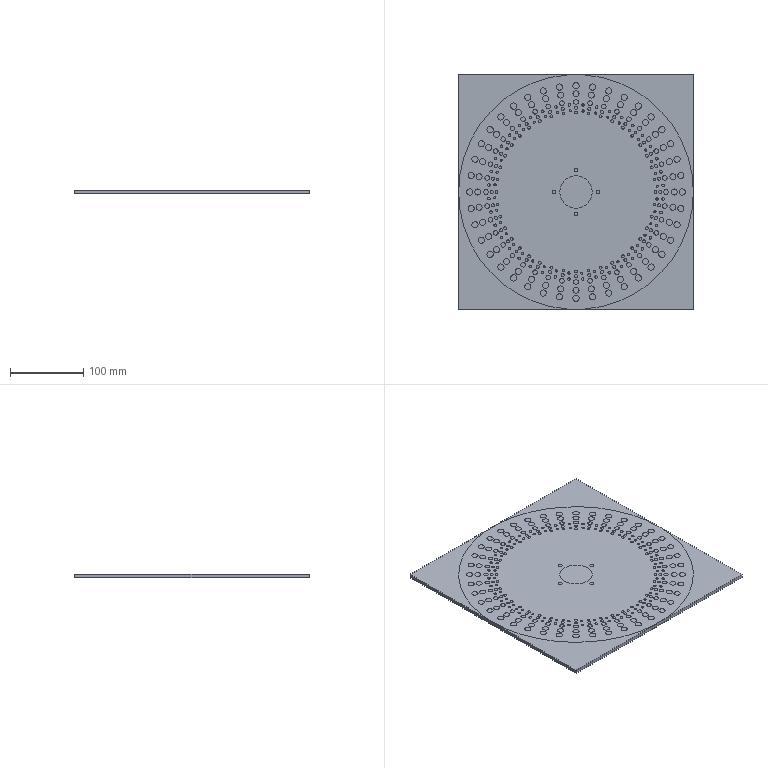NC program | NX | posted with a generic post | part box 320 x 320 x 5 mm
Lines 1 to 986 of 63198:
N10 G17 G21 G94 G90
(等高外形 , TOOL : D17R0.8圆鼻飞刀)
N12 T07 M6
N14 /M1
N16 G54
N18 G17 G0 G90 X-172.144 Y-7.615 S2000 M3
N20 G43 Z20. H7
N22 Z0.4
N24 G94 G1 Z0.2 F1600.
N26 G3 X-168.5 Y0.198 R10.2
N28 G2 X-168.486 Y2.393 R173.905 F2000.
N30 X-168.27 Y8.907 R224.797
N32 X-167.861 Y14.646 R236.128
N34 X-167.519 Y18.143 R188.644
N36 G1 X-167.43 Y18.944
N38 X-167.002 Y22.411
N40 X-166.958 Y22.734
N42 X-166.495 Y25.903
N44 X-166.42 Y26.394
N46 X-165.835 Y29.843
N48 X-165.736 Y30.384
N50 X-165.168 Y33.335
N52 X-165.023 Y34.046
N54 X-164.391 Y36.979
N56 G2 X-163.515 Y40.666 R172.039
N58 G1 X-163.504 Y40.725
N60 X-163.459 Y40.904
N62 X-162.566 Y44.32
N64 X-162.418 Y44.862
N66 X-161.528 Y47.963
N68 X-161.313 Y48.673
N70 X-160.428 Y51.514
N72 X-160.425 Y51.533
N74 X-160.217 Y52.17
N76 X-159.213 Y55.157
N78 X-159.209 Y55.177
N80 X-159.037 Y55.668
N82 X-157.73 Y59.291
N84 G2 X-155.928 Y63.842 R140.951
N86 G1 X-155.204 Y65.595
N88 X-155.198 Y65.614
N90 X-154.966 Y66.16
N92 X-153.672 Y69.114
N94 X-153.425 Y69.657
N96 X-152.087 Y72.536
N98 X-151.847 Y73.038
N100 X-150.456 Y75.861
N102 X-150.226 Y76.316
N104 X-148.47 Y79.688
N106 G2 X-144.35 Y86.927 R201.508
N108 X-141.803 Y91.008 R164.836
N110 X-140.487 Y93.026 R79.908
N112 G1 X-138.909 Y95.369
N114 X-138.905 Y95.38
N116 X-138.553 Y95.888
N118 X-136.686 Y98.533
N120 X-136.302 Y99.063
N122 X-134.557 Y101.416
N124 X-134.553 Y101.426
N126 X-134.36 Y101.682
N128 X-132.184 Y104.496
N130 X-131.82 Y104.954
N132 X-129.826 Y107.411
N134 X-129.462 Y107.85
N136 X-127.434 Y110.234
N138 X-127.424 Y110.25
N140 X-127.013 Y110.722
N142 X-124.939 Y113.058
N144 X-124.477 Y113.567
N146 X-122.385 Y115.818
N148 X-122.119 Y116.1
N150 X-119.721 Y118.569
N152 X-119.438 Y118.856
N154 X-117.036 Y121.22
N156 X-116.873 Y121.378
N158 X-114.328 Y123.778
N160 X-113.958 Y124.119
N162 X-111.454 Y126.372
N164 X-111.044 Y126.733
N166 X-108.684 Y128.759
N168 X-108.672 Y128.772
N170 X-108.129 Y129.228
N172 X-105.763 Y131.171
N174 X-105.423 Y131.445
N176 X-102.869 Y133.449
N178 X-102.857 Y133.462
N180 X-102.3 Y133.89
N182 X-99.77 Y135.786
N184 X-99.386 Y136.068
N186 X-96.741 Y137.959
N188 X-96.26 Y138.297
N190 X-93.619 Y140.095
N192 X-93.612 Y140.103
N194 X-93.228 Y140.358
N196 X-90.47 Y142.151
N198 X-90.059 Y142.412
N200 X-88.008 Y143.688
N202 G2 X-84.044 Y146.042 R227.342
N204 G1 X-83.647 Y146.271
N206 X-80.688 Y147.924
N208 X-80.15 Y148.216
N210 X-77.434 Y149.652
N212 X-76.944 Y149.905
N214 X-73.737 Y151.512
N216 G2 X-69.074 Y153.683 R141.064
N218 G1 X-68.492 Y153.941
N220 X-67.271 Y154.485
N222 X-67.253 Y154.495
N224 X-66.743 Y154.717
N226 X-63.701 Y155.993
N228 X-63.245 Y156.179
N230 X-60.241 Y157.362
N232 X-59.748 Y157.55
N234 X-56.778 Y158.641
N236 X-56.761 Y158.65
N238 X-56.25 Y158.832
N240 X-53.158 Y159.894
N242 X-52.753 Y160.029
N244 X-50.058 Y160.892
N246 X-49.256 Y161.14
N248 X-45.977 Y162.104
N250 G2 X-42.334 Y163.094 R449.314
N252 G1 X-41.678 Y163.263
N254 X-38.634 Y164.008
N256 X-38.62 Y164.014
N258 X-38.303 Y164.088
N260 X-35.011 Y164.821
N262 X-34.392 Y164.952
N264 X-31.367 Y165.55
N266 X-31.35 Y165.556
N268 X-29.346 Y165.924
N270 G2 X-26.349 Y166.42 R109.611
N272 G1 X-25.939 Y166.482
N274 X-23.845 Y166.803
N276 X-23.316 Y166.878
N278 X-20.056 Y167.3
N280 X-19.527 Y167.363
N282 X-16.394 Y167.699
N284 X-16.03 Y167.735
N286 X-12.66 Y168.022
N288 X-11.95 Y168.075
N290 X-8.871 Y168.265
N292 X-8.452 Y168.288
N294 X-5.082 Y168.422
N296 G2 X-0.103 Y168.492 R132.588
N298 G1 X2.496 Y168.48
N300 G2 X5.629 Y168.405 R104.354
N302 X9.91 Y168.207 R298.334
N304 G1 X10.54 Y168.169
N306 X13.716 Y167.937
N308 X13.735 Y167.938
N310 X15.9 Y167.75
N312 G2 X21.203 Y167.159 R243.166
N314 G1 X21.859 Y167.075
N316 X25.011 Y166.632
N318 G2 X28.508 Y166.07 R175.312
N320 G1 X29.364 Y165.921
N322 X32.912 Y165.253
N324 X33.153 Y165.205
N326 X36.068 Y164.593
N328 G2 X39.929 Y163.7 R166.413
N330 G1 X40.513 Y163.554
N332 X43.355 Y162.825
N334 X44.009 Y162.65
N336 X47.759 Y161.596
N338 G2 X51.321 Y160.493 R251.012
N340 G1 X51.338 Y160.485
N342 X54.21 Y159.538
N344 X54.229 Y159.534
N346 X54.502 Y159.441
N348 X57.853 Y158.256
N350 X57.999 Y158.203
N352 X61.943 Y156.708
N354 X64.538 Y155.651
N356 X65.27 Y155.345
N358 X68.247 Y154.059
N360 X68.784 Y153.82
N362 X71.812 Y152.429
N364 X71.989 Y152.347
N366 X75.08 Y150.847
N368 X75.633 Y150.572
N370 X78.413 Y149.139
N372 X78.427 Y149.134
N374 X78.81 Y148.933
N376 X81.67 Y147.38
N378 X81.68 Y147.377
N380 X82.256 Y147.057
N382 X85.644 Y145.119
N384 G2 X91.484 Y141.501 R211.587
N386 G1 X91.808 Y141.292
N388 X94.58 Y139.448
N390 X94.594 Y139.442
N392 G2 X100.72 Y135.083 R200.557
N394 G1 X101.134 Y134.773
N396 X103.711 Y132.8
N398 X104.049 Y132.536
N400 X106.622 Y130.474
N402 X107.11 Y130.075
N404 X109.501 Y128.067
N406 X109.878 Y127.745
N408 X112.372 Y125.557
N410 X112.792 Y125.179
N412 X115.159 Y123.006
N414 X115.483 Y122.702
N416 X117.91 Y120.37
N418 X118.27 Y120.017
N420 X120.552 Y117.724
N422 X120.815 Y117.456
N424 X123.114 Y115.042
N426 G2 X127.737 Y109.878 R173.773
N428 G1 X128.178 Y109.368
N430 X128.189 Y109.359
N432 X128.531 Y108.957
N434 X130.548 Y106.527
N436 X130.563 Y106.514
N438 X130.863 Y106.146
N440 X132.884 Y103.599
N442 X132.897 Y103.586
N444 X133.194 Y103.206
N446 X135.211 Y100.547
N448 X135.526 Y100.124
N450 X137.404 Y97.528
N452 X137.741 Y97.054
N454 X139.608 Y94.345
N456 X139.749 Y94.139
N458 X141.63 Y91.285
N460 X141.938 Y90.805
N462 X143.689 Y88.005
N464 X144.058 Y87.401
N466 X145.535 Y84.913
N468 X145.548 Y84.898
N470 G2 X147.437 Y81.571 R410.303
N472 G1 X147.721 Y81.059
N474 X149.227 Y78.246
N476 X149.234 Y78.238
N478 X149.453 Y77.818
N480 X150.903 Y74.966
N482 X151.223 Y74.321
N484 X152.566 Y71.516
N486 X152.574 Y71.505
N488 X152.892 Y70.823
N490 X154.181 Y67.97
N492 X154.337 Y67.618
N494 X155.793 Y64.204
N496 X155.929 Y63.858
N498 X156.754 Y61.806
N500 X156.889 Y61.462
N502 X157.093 Y60.94
N504 X158.353 Y57.586
N506 X158.52 Y57.125
N508 X159.581 Y54.082
N510 X159.59 Y54.065
N512 G2 X160.766 Y50.457 R468.627
N514 G1 X160.961 Y49.839
N516 X161.87 Y46.797
N518 X162.001 Y46.341
N520 X163.019 Y42.639
N522 G2 X164.585 Y36.104 R179.398
N524 G1 X164.671 Y35.71
N526 X164.767 Y35.266
N528 X165.386 Y32.224
N530 X165.392 Y32.206
N532 X165.532 Y31.477
N534 X166.075 Y28.471
N536 G2 X166.882 Y23.235 R137.906
N538 G1 X167.17 Y21.094
N540 X167.175 Y21.076
N542 X167.224 Y20.693
N544 X167.606 Y17.323
N546 X167.679 Y16.613
N548 X167.942 Y13.68
N550 X167.988 Y13.115
N552 X168.209 Y9.836
N554 X168.212 Y9.818
N556 X168.249 Y9.181
N558 X168.39 Y6.048
N560 G2 X168.478 Y-2.804 R170.816
N562 X168.216 Y-9.737 R193.369
N564 X167.34 Y-19.683 R165.071
N566 X167.17 Y-21.094 R36.699
N568 G1 X166.686 Y-24.683
N570 G2 X165.733 Y-30.385 R169.983
N572 G1 X165.524 Y-31.512
N574 G2 X165.376 Y-32.275 R41.727
N576 G1 X164.71 Y-35.537
N578 X164.67 Y-35.712
N580 X164.641 Y-35.849
N582 X163.819 Y-39.455
N584 G2 X162.071 Y-46.086 R190.1
N586 G1 X161.915 Y-46.672
N588 G2 X159.151 Y-55.353 R198.046
N590 X156.966 Y-61.269 R231.399
N592 X154.924 Y-66.249 R164.246
N594 X154.13 Y-68.081 R63.615
N596 G1 X152.905 Y-70.789
N598 X152.621 Y-71.406
N600 X151.248 Y-74.265
N602 X150.935 Y-74.904
N604 X149.514 Y-77.699
N606 X149.453 Y-77.818
N608 X147.764 Y-80.977
N610 X147.58 Y-81.315
N612 X146.264 Y-83.647
N614 X145.634 Y-84.757
N616 G2 X143.094 Y-88.961 R144.435
N618 X141.283 Y-91.808 R94.448
N620 G1 X139.996 Y-93.766
N622 X139.749 Y-94.139
N624 X137.856 Y-96.885
N626 X137.533 Y-97.346
N628 X135.299 Y-100.437
N630 G2 X130.208 Y-106.946 R181.531
N632 X121.066 Y-117.201 R175.103
N634 X115.23 Y-122.938 R189.741
N636 X111.397 Y-126.416 R144.753
N638 X108.184 Y-129.177 R136.374
N640 X103.274 Y-133.142 R188.011
N642 X95.198 Y-139.027 R178.208
N644 G1 X95.042 Y-139.146
N646 G2 X88.301 Y-143.507 R195.218
N648 X84.544 Y-145.748 R120.532
N650 G1 X82.03 Y-147.184
N652 X81.78 Y-147.32
N654 X78.353 Y-149.182
N656 G2 X70.899 Y-152.859 R204.711
N658 X64.12 Y-155.823 R194.388
N660 X57.203 Y-158.493 R193.422
N662 G1 X54.551 Y-159.425
N664 X54.229 Y-159.532
N666 X51.32 Y-160.492
N668 X51.017 Y-160.591
N670 X47.03 Y-161.809
N672 G2 X40.513 Y-163.553 R192.449
N674 G1 X39.929 Y-163.699
N676 G2 X24.843 Y-166.661 R171.978
N678 X17.537 Y-167.582 R186.734
N680 G1 X17.519 Y-167.586
N682 X17.196 Y-167.618
N684 X14.86 Y-167.84
N686 X14.281 Y-167.892
N688 X10.534 Y-168.169
N690 X10.201 Y-168.189
N692 X6.581 Y-168.372
N694 G2 X-0.583 Y-168.496 R185.696
N696 X-11.272 Y-168.121 R170.89
N698 G1 X-12.532 Y-168.03
N700 X-16.361 Y-167.709
N702 G2 X-20.709 Y-167.215 R137.564
N704 G1 X-23.316 Y-166.877
N706 X-23.845 Y-166.801
N708 X-26.832 Y-166.347
N710 G2 X-30.22 Y-165.765 R99.167
N712 X-31.317 Y-165.56 R48.578
N714 G1 X-34.264 Y-164.976
N716 X-34.683 Y-164.89
N718 X-37.889 Y-164.181
N720 X-38.303 Y-164.088
N722 X-41.949 Y-163.196
N724 G2 X-47.178 Y-161.753 R154.378
N726 X-51.509 Y-160.43 R137.571
N728 X-55.998 Y-158.919 R184.503
N730 G1 X-56.542 Y-158.728
N732 X-60.298 Y-157.348
N734 G2 X-66.638 Y-154.76 R213.521
N736 G1 X-67.035 Y-154.59
N738 X-69.976 Y-153.279
N740 X-70.479 Y-153.05
N742 X-73.374 Y-151.682
N744 X-73.738 Y-151.508
N746 X-77.41 Y-149.672
N748 G2 X-83.837 Y-146.16 R195.638
N750 X-88.545 Y-143.353 R146.538
N752 X-90.83 Y-141.915 R94.043
N754 X-94.305 Y-139.631 R119.24
N756 X-97.071 Y-137.722 R99.319
N758 G1 X-99.86 Y-135.728
N760 G2 X-105.596 Y-131.305 R202.464
N762 X-110.992 Y-126.776 R181.83
N764 G1 X-111.336 Y-126.475
N766 X-113.752 Y-124.304
N768 X-114.229 Y-123.868
N770 X-117.092 Y-121.176
N772 G2 X-119.72 Y-118.568 R128.824
N774 G1 X-121.835 Y-116.393
N776 X-122.119 Y-116.099
N778 X-124.453 Y-113.59
N780 X-124.651 Y-113.375
N782 X-127.419 Y-110.266
N784 G2 X-130.733 Y-106.296 R163.491
N786 X-134.068 Y-102.063 R155.524
N788 G1 X-134.36 Y-101.682
N790 X-136.739 Y-98.47
N792 G2 X-139.367 Y-94.692 R143.743
N794 X-142.61 Y-89.741 R152.771
N796 G1 X-143.098 Y-88.963
N798 X-143.69 Y-88.012
N800 X-144.271 Y-87.048
N802 G2 X-146.522 Y-83.201 R146.461
N804 G1 X-146.847 Y-82.627
N806 X-148.542 Y-79.548
N808 G2 X-153.666 Y-69.137 R178.34
N810 X-156.324 Y-62.881 R168.943
N812 G1 X-156.51 Y-62.421
N814 X-157.932 Y-58.746
N816 G2 X-159.816 Y-53.378 R171.202
N818 X-160.666 Y-50.773 R307.14
N820 G1 X-161.171 Y-49.148
N822 X-161.397 Y-48.438
N824 G2 X-163.494 Y-40.761 R195.383
N826 X-166.004 Y-28.907 R174.3
N828 G1 X-166.398 Y-26.522
N830 X-166.418 Y-26.397
N832 X-166.445 Y-26.297
N834 G2 X-167.192 Y-20.897 R164.368
N836 X-167.783 Y-15.483 R149.509
N838 G1 X-167.841 Y-14.864
N840 X-168.109 Y-11.451
N842 G2 X-168.5 Y0.198 R173.905
N844 G1 X-168.497
N846 X-168.495 Y0.49
N848 X-168.491 Y0.781
N850 X-168.466 Y3.113
N852 X-168.464 Y3.404
N854 X-168.457 Y3.696
N856 X-168.45 Y3.987
N858 X-168.442 Y4.279
N860 X-168.434 Y4.57
N862 X-168.425 Y4.861
N864 X-168.417 Y5.153
N866 X-168.408 Y5.444
N868 X-168.398 Y5.735 Z0.199
N870 X-168.388 Y6.027
N872 X-168.378 Y6.318
N874 X-168.368 Y6.609
N876 X-168.357 Y6.901
N878 X-168.346 Y7.192
N880 X-168.334 Y7.483
N882 X-168.322 Y7.774
N884 X-168.31 Y8.066
N886 X-168.298 Y8.357
N888 X-168.285 Y8.648
N890 X-168.269 Y8.939
N892 X-168.252 Y9.23
N894 X-168.234 Y9.521
N896 X-168.215 Y9.812
N898 X-168.197 Y10.103
N900 X-168.178 Y10.394
N902 X-168.159 Y10.685
N904 X-168.139 Y10.975
N906 X-168.119 Y11.266
N908 X-168.099 Y11.557
N910 X-168.078 Y11.848
N912 X-168.057 Y12.139
N914 X-168.035 Y12.429
N916 X-168.014 Y12.72
N918 X-167.992 Y13.011
N920 X-167.969 Y13.301
N922 X-167.946 Y13.592
N924 X-167.923 Y13.882
N926 X-167.9 Y14.173
N928 X-167.876 Y14.463
N930 X-167.851 Y14.754
N932 X-167.825 Y15.044
N934 X-167.799 Y15.334
N936 X-167.772 Y15.625
N938 X-167.744 Y15.915
N940 X-167.716 Y16.205 Z0.198
N942 X-167.688 Y16.495
N944 X-167.659 Y16.785
N946 X-167.63 Y17.075
N948 X-167.601 Y17.365
N950 X-167.571 Y17.655
N952 X-167.54 Y17.945
N954 X-167.509 Y18.235
N956 X-167.444 Y18.814
N958 X-167.41 Y19.104
N960 X-167.017 Y22.286
N962 X-166.979 Y22.575
N964 X-166.939 Y22.864
N966 X-166.518 Y25.748
N968 X-166.475 Y26.036
N970 X-166.431 Y26.325
N972 X-166.383 Y26.612 Z0.197
N974 X-165.847 Y29.773
N976 X-165.795 Y30.06
N978 X-165.743 Y30.347
N980 X-165.688 Y30.633
N982 X-165.192 Y33.21
N984 X-165.135 Y33.495
N986 X-165.077 Y33.781
N988 X-165.019 Y34.067
N990 X-164.404 Y36.916
N992 X-164.34 Y37.2 Z0.196
N994 X-164.274 Y37.484
N996 X-164.208 Y37.768
N998 X-164.142 Y38.052
N1000 X-164.076 Y38.336
N1002 X-164.009 Y38.62
N1004 X-163.942 Y38.903
N1006 X-163.874 Y39.187
N1008 X-163.806 Y39.47
N1010 X-163.738 Y39.754
N1012 X-163.67 Y40.037
N1014 X-163.601 Y40.32
N1016 X-163.531 Y40.604
N1018 X-163.463 Y40.887
N1020 X-163.39 Y41.169
N1022 X-162.578 Y44.271
N1024 X-162.502 Y44.552
N1026 X-162.425 Y44.834
N1028 X-162.345 Y45.114
N1030 X-161.542 Y47.916 Z0.195
N1032 X-161.458 Y48.195
N1034 X-161.374 Y48.474
N1036 X-161.288 Y48.753
N1038 X-160.508 Y51.258
N1040 X-160.424 Y51.536
N1042 X-160.243 Y52.091
N1044 X-160.151 Y52.367
N1046 X-159.225 Y55.131
N1048 X-159.129 Y55.406
N1050 X-159.032 Y55.681
N1052 X-157.747 Y59.246 Z0.194
N1054 X-157.644 Y59.519
N1056 X-157.541 Y59.792
N1058 X-157.437 Y60.064
N1060 X-157.333 Y60.336
N1062 X-157.228 Y60.608
N1064 X-157.122 Y60.88
N1066 X-157.016 Y61.151
N1068 X-156.909 Y61.422
N1070 X-156.802 Y61.693
N1072 X-156.694 Y61.964
N1074 X-156.585 Y62.235
N1076 X-156.476 Y62.505
N1078 X-156.367 Y62.775
N1080 X-156.257 Y63.045
N1082 X-156.146 Y63.315
N1084 X-156.035 Y63.584
N1086 X-155.923 Y63.853
N1088 X-155.255 Y65.47
N1090 X-155.145 Y65.74
N1092 X-155.031 Y66.008
N1094 X-154.916 Y66.275
N1096 X-153.746 Y68.945 Z0.193
N1098 X-153.628 Y69.212
N1100 X-153.507 Y69.477
N1102 X-153.386 Y69.742
N1104 X-152.157 Y72.386
N1106 X-152.033 Y72.649
N1108 X-151.907 Y72.912
N1110 X-151.78 Y73.174
N1112 X-150.489 Y75.788
N1114 X-150.36 Y76.049
N1116 X-150.229 Y76.31
N1118 X-150.095 Y76.568
N1120 X-148.479 Y79.671 Z0.192
N1122 X-148.34 Y79.927
N1124 X-148.201 Y80.183
N1126 X-148.061 Y80.439
N1128 X-147.921 Y80.694
N1130 X-147.78 Y80.95
N1132 X-147.639 Y81.205
N1134 X-147.498 Y81.46
N1136 X-147.356 Y81.714
N1138 X-147.214 Y81.969
N1140 X-147.072 Y82.223
N1142 X-146.929 Y82.477
N1144 X-146.786 Y82.731
N1146 X-146.642 Y82.985
N1148 X-146.498 Y83.239
N1150 X-146.354 Y83.492
N1152 X-146.21 Y83.745
N1154 X-146.065 Y83.998
N1156 X-145.919 Y84.251
N1158 X-145.774 Y84.503
N1160 X-145.628 Y84.755
N1162 X-145.481 Y85.007
N1164 X-145.334 Y85.259
N1166 X-145.187 Y85.511
N1168 X-145.04 Y85.762
N1170 X-144.892 Y86.013 Z0.191
N1172 X-144.744 Y86.264
N1174 X-144.595 Y86.515
N1176 X-144.446 Y86.766
N1178 X-144.296 Y87.016
N1180 X-144.145 Y87.265
N1182 X-143.993 Y87.514
N1184 X-143.841 Y87.763
N1186 X-143.689 Y88.011
N1188 X-143.536 Y88.259
N1190 X-143.383 Y88.507
N1192 X-143.229 Y88.755
N1194 X-143.075 Y89.002
N1196 X-142.92 Y89.249
N1198 X-142.765 Y89.496
N1200 X-142.61 Y89.743
N1202 X-142.454 Y89.989
N1204 X-142.298 Y90.235
N1206 X-142.141 Y90.481
N1208 X-141.984 Y90.727
N1210 X-141.826 Y90.972
N1212 X-141.67 Y91.218
N1214 X-141.514 Y91.464
N1216 X-141.357 Y91.71
N1218 X-141.198 Y91.954
N1220 X-141.039 Y92.198
N1222 X-140.879 Y92.442
N1224 X-140.717 Y92.685
N1226 X-140.555 Y92.926
N1228 X-138.926 Y95.344 Z0.19
N1230 X-138.763 Y95.585
N1232 X-138.597 Y95.825
N1234 X-138.429 Y96.063
N1236 X-136.748 Y98.445
N1238 X-136.578 Y98.682
N1240 X-136.407 Y98.918
N1242 X-136.235 Y99.153
N1244 X-134.675 Y101.262
N1246 X-134.501 Y101.496
N1248 X-134.325 Y101.728
N1250 X-132.185 Y104.495 Z0.189
N1252 X-132.003 Y104.723
N1254 X-131.822 Y104.951
N1256 X-131.638 Y105.178
N1258 X-129.985 Y107.215
N1260 X-129.801 Y107.441
N1262 X-129.615 Y107.665
N1264 X-129.429 Y107.889
N1266 X-127.542 Y110.111
N1268 X-127.352 Y110.332
N1270 X-127.161 Y110.552
N1272 X-126.969 Y110.772
N1274 X-125.033 Y112.951 Z0.188
N1276 X-124.838 Y113.168
N1278 X-124.642 Y113.384
N1280 X-124.446 Y113.599
N1282 X-122.46 Y115.733
N1284 X-122.263 Y115.947
N1286 X-122.062 Y116.159
N1288 X-119.828 Y118.459
N1290 X-119.624 Y118.667
N1292 X-119.419 Y118.874
N1294 X-117.134 Y121.124 Z0.187
N1296 X-116.925 Y121.327
N1298 X-116.715 Y121.529
N1300 X-116.504 Y121.73
N1302 X-114.381 Y123.728
N1304 X-114.167 Y123.926
N1306 X-113.953 Y124.123
N1308 X-111.569 Y126.268
N1310 X-111.352 Y126.462
N1312 X-111.133 Y126.654 Z0.186
N1314 X-110.913 Y126.845
N1316 X-108.701 Y128.744
N1318 X-108.48 Y128.934
N1320 X-108.257 Y129.121
N1322 X-108.032 Y129.308
N1324 X-105.78 Y131.158
N1326 X-105.553 Y131.341
N1328 X-105.325 Y131.522
N1330 X-103.033 Y133.324 Z0.185
N1332 X-102.804 Y133.503
N1334 X-102.341 Y133.859
N1336 X-102.109 Y134.034
N1338 X-99.776 Y135.782
N1340 X-99.541 Y135.954
N1342 X-99.305 Y136.126
N1344 X-96.934 Y137.821
N1346 X-96.697 Y137.991
N1348 X-96.458 Y138.158
N1350 X-96.219 Y138.325
N1352 X-93.811 Y139.967 Z0.184
N1354 X-93.57 Y140.131
N1356 X-93.327 Y140.293
N1358 X-93.084 Y140.453
N1360 X-90.639 Y142.041
N1362 X-90.395 Y142.199
N1364 X-90.149 Y142.356
N1366 X-89.902 Y142.51
N1368 X-88.169 Y143.588
N1370 X-87.921 Y143.741
N1372 X-87.671 Y143.892
N1374 X-87.422 Y144.043
N1376 X-87.172 Y144.193
N1378 X-86.923 Y144.343
N1380 X-86.672 Y144.493
N1382 X-86.422 Y144.643
N1384 X-86.172 Y144.792
N1386 X-85.921 Y144.941
N1388 X-85.67 Y145.089
N1390 X-85.419 Y145.238 Z0.183
N1392 X-85.168 Y145.386
N1394 X-84.917 Y145.533
N1396 X-84.665 Y145.68
N1398 X-84.414 Y145.827
N1400 X-84.162 Y145.974
N1402 X-83.909 Y146.12
N1404 X-83.657 Y146.265
N1406 X-83.402 Y146.408
N1408 X-80.857 Y147.829
N1410 X-80.602 Y147.97
N1412 X-80.346 Y148.109
N1414 X-80.09 Y148.248
N1416 X-77.513 Y149.61
N1418 X-77.254 Y149.745
N1420 X-76.995 Y149.878
N1422 X-76.735 Y150.01
N1424 X-74.129 Y151.315 Z0.182
N1426 X-73.867 Y151.444
N1428 X-73.605 Y151.572
N1430 X-73.343 Y151.699
N1432 X-70.707 Y152.944
N1434 X-70.443 Y153.067
N1436 X-70.178 Y153.189
N1438 X-67.517 Y154.377
N1440 X-67.25 Y154.496
N1442 X-66.983 Y154.612
N1444 X-66.715 Y154.728 Z0.181
N1446 X-63.759 Y155.969
N1448 X-63.489 Y156.08
N1450 X-63.219 Y156.189
N1452 X-60.507 Y157.257
N1454 X-60.236 Y157.364
N1456 X-59.963 Y157.468
N1458 X-59.691 Y157.571
N1460 X-56.955 Y158.576
N1462 X-56.682 Y158.679 Z0.18
N1464 X-56.407 Y158.777
N1466 X-56.132 Y158.873
N1468 X-53.375 Y159.819
N1470 X-53.099 Y159.913
N1472 X-52.823 Y160.006
N1474 X-52.545 Y160.095
N1476 X-50.324 Y160.807
N1478 X-50.047 Y160.895
N1480 X-49.49 Y161.068
N1482 X-49.211 Y161.153
N1484 X-46.135 Y162.058 Z0.179
N1486 X-45.855 Y162.138
N1488 X-45.574 Y162.216
N1490 X-45.293 Y162.293
N1492 X-45.012 Y162.37
N1494 X-44.731 Y162.447
N1496 X-44.449 Y162.523
N1498 X-44.168 Y162.6
N1500 X-43.887 Y162.676
N1502 X-43.605 Y162.752
N1504 X-43.324 Y162.828
N1506 X-43.042 Y162.904
N1508 X-42.761 Y162.98
N1510 X-42.479 Y163.055
N1512 X-42.197 Y163.129
N1514 X-41.915 Y163.202
N1516 X-41.633 Y163.274
N1518 X-38.801 Y163.967
N1520 X-38.519 Y164.038
N1522 X-38.235 Y164.103
N1524 X-35.105 Y164.8 Z0.178
N1526 X-34.82 Y164.861
N1528 X-34.535 Y164.922
N1530 X-34.249 Y164.98
N1532 X-31.39 Y165.546
N1534 X-31.104 Y165.601
N1536 X-29.384 Y165.917
N1538 X-29.097 Y165.969
N1540 X-28.81 Y166.019
N1542 X-28.522 Y166.069
N1544 X-28.235 Y166.118
N1546 X-27.947 Y166.166
N1548 X-27.66 Y166.214
N1550 X-27.372 Y166.26
N1552 X-27.084 Y166.306
N1554 X-26.796 Y166.351
N1556 X-26.508 Y166.396
N1558 X-26.22 Y166.44
N1560 X-25.932 Y166.483 Z0.177
N1562 X-23.915 Y166.792
N1564 X-23.626 Y166.834
N1566 X-23.338 Y166.875
N1568 X-23.049 Y166.913
N1570 X-20.158 Y167.287
N1572 X-19.869 Y167.323
N1574 X-19.579 Y167.357
N1576 X-19.289 Y167.389
N1578 X-16.681 Y167.668
N1580 X-16.391 Y167.699
N1582 X-16.101 Y167.728
N1584 X-15.811 Y167.754
N1586 X-12.906 Y168.001 Z0.176
N1588 X-12.616 Y168.026
N1590 X-12.034 Y168.068
N1592 X-11.744 Y168.087
N1594 X-9.125 Y168.249
N1596 X-8.834 Y168.267
N1598 X-8.543 Y168.283
N1600 X-8.252 Y168.296
N1602 X-5.339 Y168.412
N1604 X-5.048 Y168.423 Z0.175
N1606 X-4.757 Y168.432
N1608 X-4.465 Y168.441
N1610 X-4.174 Y168.449
N1612 X-3.882 Y168.456
N1614 X-3.591 Y168.463
N1616 X-3.3 Y168.469
N1618 X-3.008 Y168.474
N1620 X-2.717 Y168.479
N1622 X-2.425 Y168.483
N1624 X-2.134 Y168.486
N1626 X-1.842 Y168.489
N1628 X-1.551 Y168.491
N1630 X-1.259 Y168.492
N1632 X-0.968 Y168.493
N1634 X-0.676 Y168.494
N1636 X-0.385 Y168.493
N1638 X-0.093 Y168.492
N1640 X2.239 Y168.481
N1642 X2.53 Y168.48
N1644 X2.822 Y168.476
N1646 X3.113 Y168.473
N1648 X3.404 Y168.468
N1650 X3.696 Y168.462
N1652 X3.987 Y168.456
N1654 X4.279 Y168.449
N1656 X4.57 Y168.441
N1658 X4.861 Y168.432
N1660 X5.153 Y168.422
N1662 X5.444 Y168.412
N1664 X5.735 Y168.401 Z0.174
N1666 X6.027 Y168.389
N1668 X6.318 Y168.377
N1670 X6.609 Y168.365
N1672 X6.9 Y168.352
N1674 X7.192 Y168.34
N1676 X7.483 Y168.327
N1678 X7.774 Y168.313
N1680 X8.065 Y168.3
N1682 X8.356 Y168.286
N1684 X8.647 Y168.272
N1686 X8.939 Y168.257
N1688 X9.23 Y168.242
N1690 X9.521 Y168.227
N1692 X9.812 Y168.212
N1694 X10.103 Y168.195
N1696 X10.394 Y168.178
N1698 X10.685 Y168.159
N1700 X13.592 Y167.946
N1702 X13.883 Y167.925
N1704 X15.044 Y167.825
N1706 X15.334 Y167.799
N1708 X17.365 Y167.601 Z0.173
N1710 X17.655 Y167.571
N1712 X17.945 Y167.54
N1714 X18.235 Y167.509
N1716 X21.13 Y167.165
N1718 X21.419 Y167.132
N1720 X21.708 Y167.094
N1722 X21.997 Y167.056
N1724 X24.884 Y166.65
N1726 X25.172 Y166.608
N1728 X25.46 Y166.564
N1730 X25.748 Y166.519
N1732 X26.036 Y166.475
N1734 X26.324 Y166.429
N1736 X26.612 Y166.383 Z0.172
N1738 X26.9 Y166.337
N1740 X27.188 Y166.29
N1742 X27.475 Y166.243
N1744 X27.763 Y166.196
N1746 X28.05 Y166.147
N1748 X28.338 Y166.099
N1750 X28.625 Y166.049
N1752 X29.199 Y165.95
N1754 X29.486 Y165.898
N1756 X32.637 Y165.305
N1758 X32.924 Y165.251
N1760 X36.062 Y164.594
N1762 X36.347 Y164.532
N1764 X36.632 Y164.469
N1766 X36.916 Y164.405
N1768 X37.2 Y164.341 Z0.171
N1770 X37.485 Y164.277
N1772 X37.769 Y164.212
N1774 X38.053 Y164.146
N1776 X38.337 Y164.08
N1778 X38.621 Y164.013
N1780 X38.904 Y163.946
N1782 X39.188 Y163.879
N1784 X39.471 Y163.811
N1786 X39.755 Y163.742
N1788 X40.038 Y163.673
N1790 X40.32 Y163.602
N1792 X40.603 Y163.531
N1794 X43.144 Y162.879
N1796 X43.426 Y162.806
N1798 X43.99 Y162.655
N1800 X44.27 Y162.576
N1802 X47.638 Y161.63 Z0.17
N1804 X47.917 Y161.548
N1806 X48.196 Y161.464
N1808 X48.475 Y161.379
N1810 X48.754 Y161.294
N1812 X49.033 Y161.208
N1814 X49.311 Y161.123
N1816 X49.59 Y161.036
N1818 X49.868 Y160.95
N1820 X50.147 Y160.863
N1822 X50.425 Y160.776
N1824 X50.703 Y160.689
N1826 X50.981 Y160.601
N1828 X51.259 Y160.513
N1830 X51.535 Y160.42
N1832 X54.026 Y159.598
N1834 X54.303 Y159.509
N1836 X54.579 Y159.414
N1838 X58.427 Y158.053 Z0.169
N1840 X58.7 Y157.951
N1842 X58.972 Y157.848
N1844 X59.245 Y157.745
N1846 X59.517 Y157.642
N1848 X59.79 Y157.538
N1850 X60.062 Y157.433
N1852 X60.334 Y157.329
N1854 X60.606 Y157.224
N1856 X60.878 Y157.118
N1858 X61.149 Y157.012
N1860 X61.421 Y156.906
N1862 X61.692 Y156.8
N1864 X61.963 Y156.693
N1866 X62.234 Y156.585
N1868 X62.505 Y156.478
N1870 X62.775 Y156.369
N1872 X64.395 Y155.71
N1874 X64.665 Y155.598
N1876 X65.202 Y155.373
N1878 X65.47 Y155.258
N1880 X68.146 Y154.102 Z0.168
N1882 X68.413 Y153.985
N1884 X68.679 Y153.866
N1886 X68.945 Y153.746
N1888 X71.594 Y152.53
N1890 X71.859 Y152.408
N1892 X72.122 Y152.283
N1894 X75.007 Y150.883
N1896 X75.268 Y150.754
N1898 X75.529 Y150.624
N1900 X75.789 Y150.491
N1902 X78.38 Y149.156 Z0.167
N1904 X78.639 Y149.023
N1906 X78.896 Y148.886
N1908 X81.459 Y147.497
N1910 X81.715 Y147.358
N1912 X82.225 Y147.075
N1914 X82.478 Y146.93
N1916 X85.514 Y145.193
N1918 X85.766 Y145.046
N1920 X86.016 Y144.896 Z0.166
N1922 X86.266 Y144.746
N1924 X86.515 Y144.596
N1926 X86.765 Y144.445
N1928 X87.014 Y144.294
N1930 X87.263 Y144.142
N1932 X87.512 Y143.99
N1934 X87.76 Y143.838
N1936 X88.009 Y143.685
N1938 X88.257 Y143.533
N1940 X88.505 Y143.379
N1942 X88.753 Y143.226
N1944 X89. Y143.072
N1946 X89.247 Y142.918
N1948 X89.495 Y142.763
N1950 X89.741 Y142.608
N1952 X89.988 Y142.453
N1954 X90.235 Y142.297
N1956 X90.481 Y142.141
N1958 X90.727 Y141.985
N1960 X90.973 Y141.828
N1962 X91.218 Y141.671
N1964 X91.464 Y141.514
N1966 X91.709 Y141.356
N1968 X91.952 Y141.196
N1970 X94.379 Y139.581